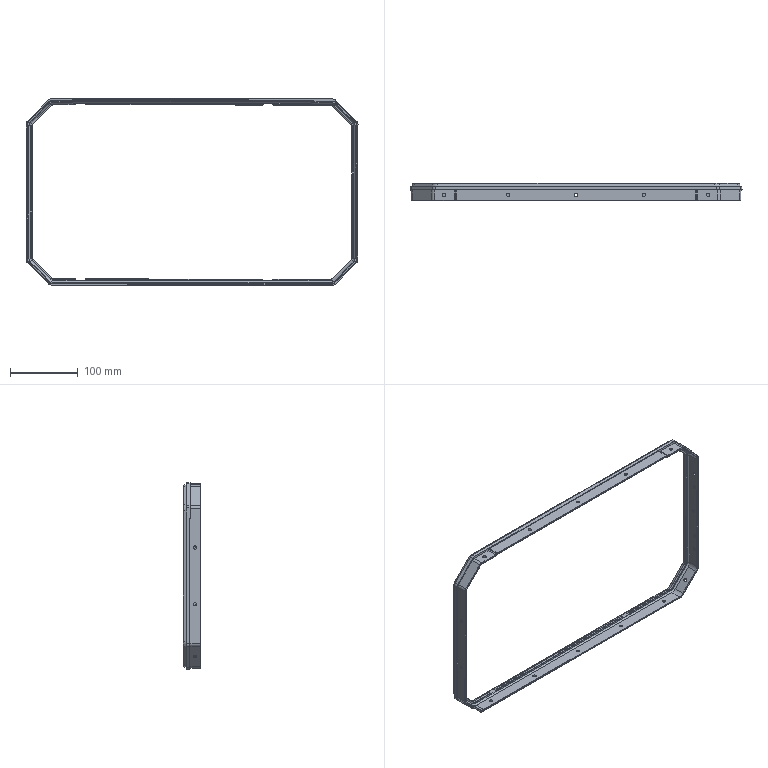Part | SolidWorks | features BaseBody 1 | 1 solid | 399 faces | box 490.167 x 26.135 x 275.35 mm | volume 141245 mm3 | cylinder 147 | plane 120 | torus 56 | cone 52 | sphere 16 | spline 8 | commonest cylinder face diameters 1 x61 4.9 x38 12 x16 5.2 x8 10.6 x8 21 x8